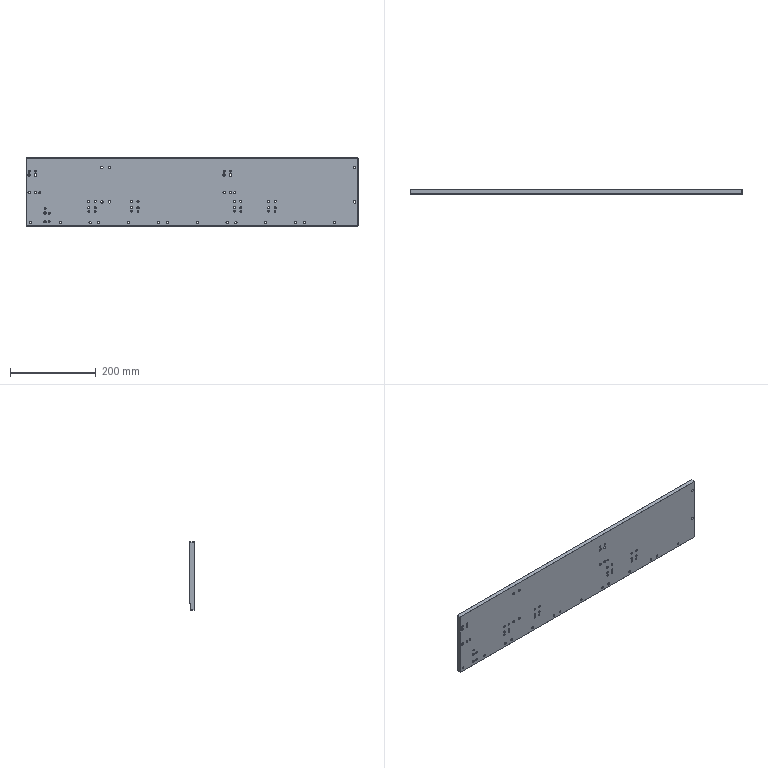Part | NX | 1 solid | 282 faces | box 775 x 10 x 159 mm | volume 1200047 mm3 | cylinder 138 | cone 114 | plane 30 | commonest cylinder face diameters 5 x60 4 x34 5.5 x16 6 x12 10 x12 4.2 x4